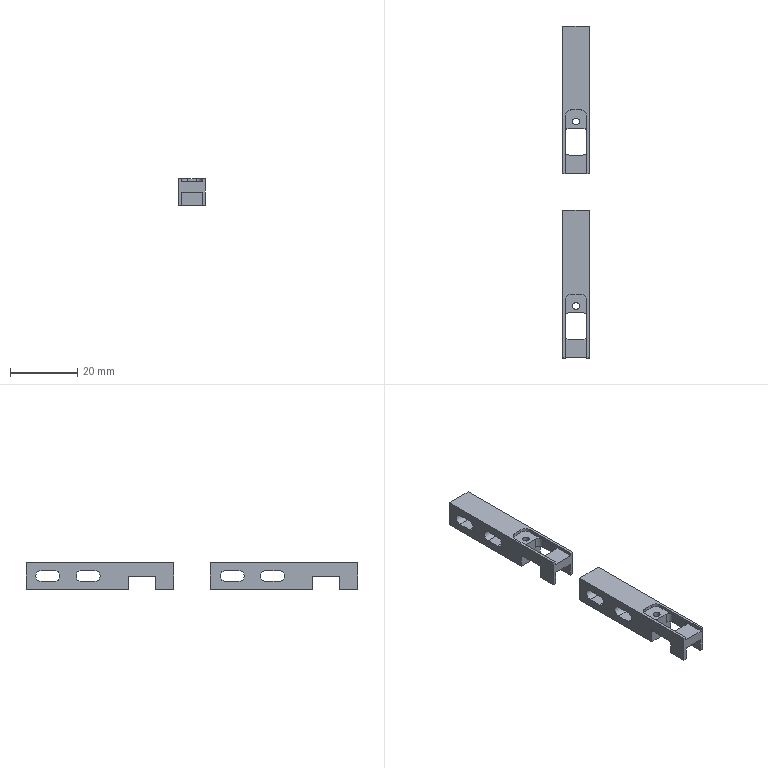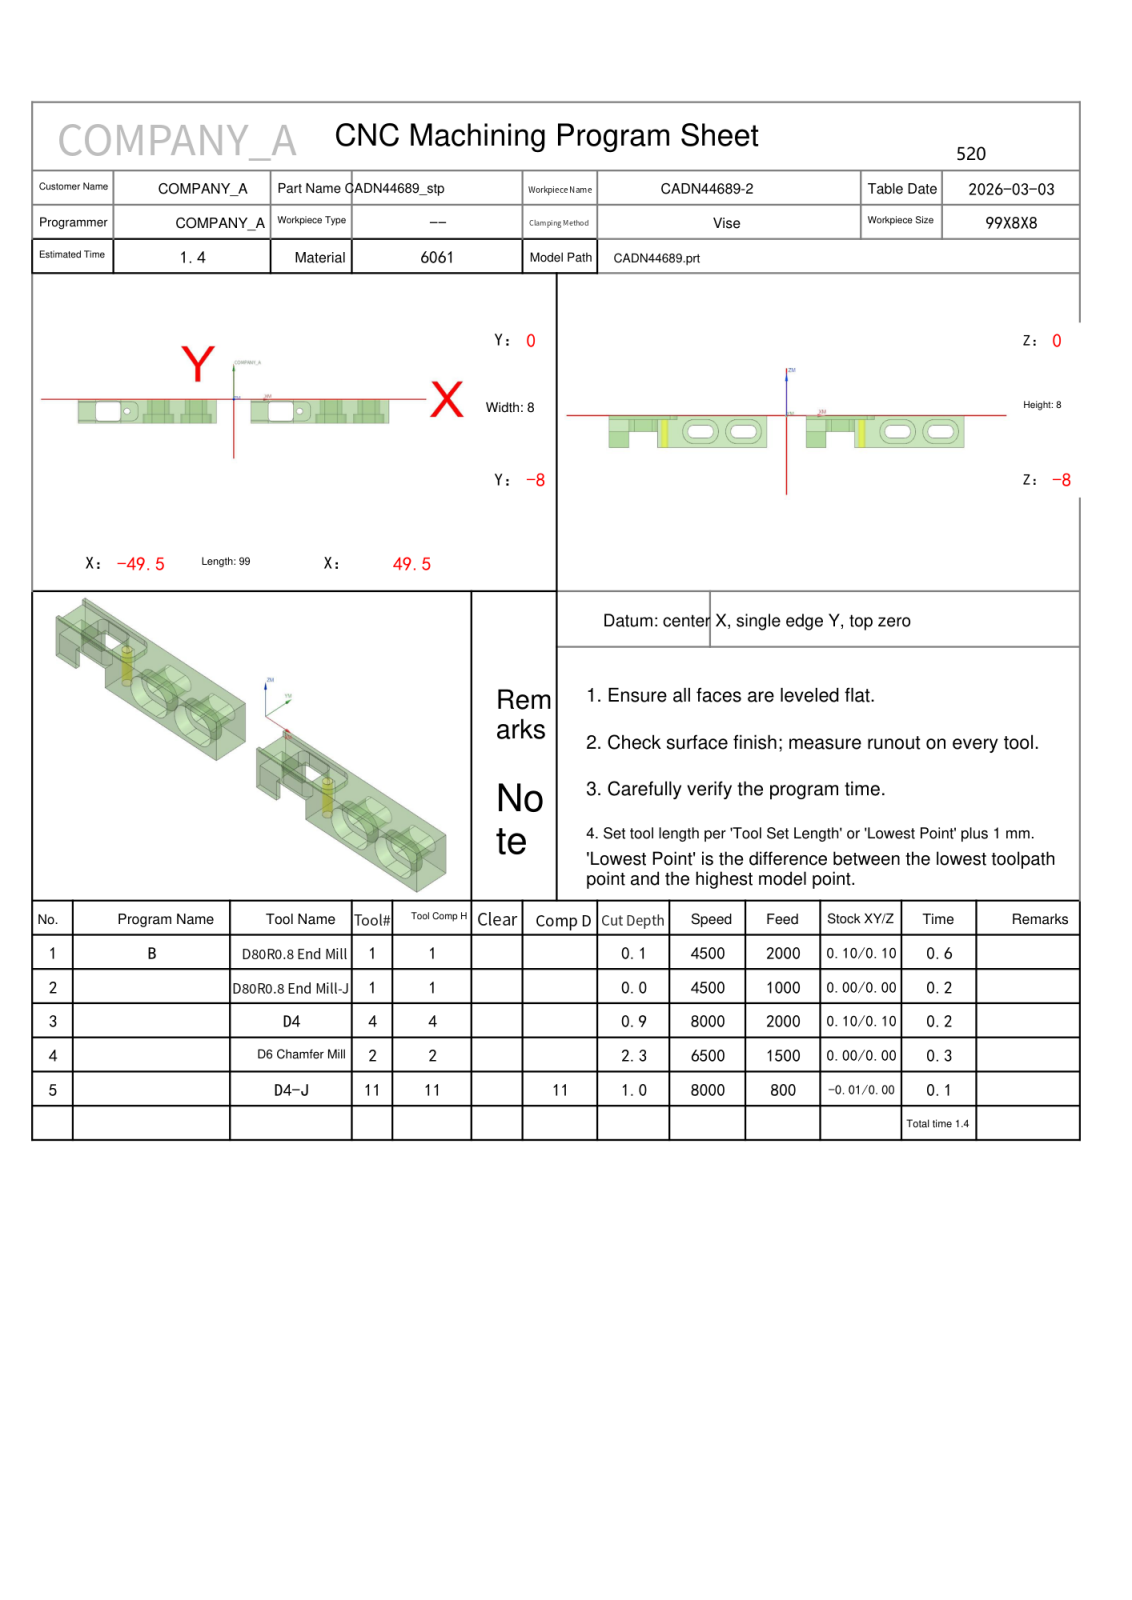NC program | NX | posted by the shop | part box 8 x 99 x 8 mm
Whole program:
%
O0001
(Machine time: 2.46 MIN)
(===Total Tool:4===)
(T1=D80R0.8 Indexable End Mill D=80.  R=0.8  D-  H01 Z=0.    )
(T4=D4      D=4.   R=0.   D-  H04 Z=-0.9  )
(T2=D6 Chamfer Mill   D=6.   R=0.   D-  H02 Z=-2.33 )
(T11=D4-J   D=4.   R=0.   D11 H11 Z=-1.   )
G80 G90 G17 G49 G40
G91 G28 Z0
M01
N1 T01 M06
(D80R0.8 Indexable End Mill  D=80. R=0.8 H=01 ce=0.10 di=0.10)
G00 G90 G54 X-101.597 Y-4. M03 S4500
G43 H01 Z50.
M08
Z5.62
G01 Z3.62 F2000.
X-89.597
X89.597
X101.597
Z5.62
G00 X-101.597
Z4.74
G01 Z2.74
X-89.597
X89.597
X101.597
Z4.74
G00 Z50.
X-101.597
Z3.86
G01 Z1.86
X-89.597
X89.597
X101.597
Z3.86
G00 Z50.
X-101.597
Z2.98
G01 Z.98
X-89.597
X89.597
X101.597
Z2.98
G00 Z50.
X-101.597
Z2.1
G01 Z.1
X-89.597
X89.597
X101.597
Z2.1
G00 Z50.
G91 G28 Z0.0
M05
M09
G91 G28 Z0.0
M01
N2 T01 M06
(D80R0.8 Indexable End Mill-J  D=80. R=0.8 H=01 ce=0.00 di=0.00)
G00 G90 G54 X-101.499 Y-4. M03 S4500
G43 H01 Z50.
M08
Z2.
G01 Z0.0 F1000.
X-89.499
X89.499
X101.499
Z2.
G00 Z50.
G91 G28 Z0.0
M05
M09
G91 G28 Z0.0
M01
N3 T04 M06
(D4  D=4. R=0. H=04 ce=0.10 di=0.10)
G00 G90 G54 X-54.6 Y-5.15 M03 S8000
G43 H04 Z11.8
M08
Z1.2
G01 Z-.3 F2000.
X-51.46
X-32.6
Y-2.85
X-51.46
X-54.6
Z1.2
G00 Y-5.15
Z.9
G01 Z-.6
X-51.46
X-32.6
Y-2.85
X-51.46
X-54.6
Z.9
G00 Y-5.15
Z.6
G01 Z-.9
X-51.46
X-32.6
Y-2.85
X-51.46
X-54.6
Z.6
G00 Z11.8
X.4 Y-5.15
Z1.2
G01 Z-.3
X3.54
X22.4
Y-2.85
X3.54
X.4
Z1.2
G00 Y-5.15
Z.9
G01 Z-.6
X3.54
X22.4
Y-2.85
X3.54
X.4
Z.9
G00 Y-5.15
Z.6
G01 Z-.9
X3.54
X22.4
Y-2.85
X3.54
X.4
Z.6
G00 Z11.8
G91 G28 Z0.0
M05
M09
G91 G28 Z0.0
M01
N4 T02 M06
(D6 Chamfer Mill  D=6. R=0. H=02 ce=0.00 di=0.10)
G00 G90 G54 X-34. Y-4. M03 S5000
G43 H02 Z50.
M08
G98 G81 X-34. Y-4. Z-2.325 R2. F150.
X21.
G80
G00 Z50.
G00 G90 X27.886 Y-8.827 M03 S6500
Z50.
Z.572
G01 Z-.8 F1500.
G03 X27.6 Y-8.627 I-1.286 J-1.532
G01 X27.554 Y-8.597
X27.5 Y-8.6
X5.5
G02 X4.9 Y-8. I0.0 J.6
G01 Y-7.25
G02 X5.5 Y-6.65 I.6 J0.0
G01 X22.5
G03 X23.9 Y-5.25 I0.0 J1.4
G01 Y-2.75
G03 X22.5 Y-1.35 I-1.4 J0.0
G01 X5.5
G02 X4.9 Y-.75 I0.0 J.6
G01 Y0.0
G02 X5.5 Y.6 I.6 J0.0
G01 X49.5
G02 X50.1 Y0.0 I0.0 J-.6
G01 Y-8.
G02 X49.5 Y-8.6 I-.6 J0.0
G01 X27.5
X27.446 Y-8.597
X27.4 Y-8.627
G03 X27.114 Y-8.827 I1. J-1.732
G01 Z.572
G00 Z10.
X-27.114
Z.572
G01 Z-.8
G03 X-27.4 Y-8.627 I-1.286 J-1.532
G01 X-27.446 Y-8.597
X-27.5 Y-8.6
X-49.5
G02 X-50.1 Y-8. I0.0 J.6
G01 Y-7.25
G02 X-49.5 Y-6.65 I.6 J0.0
G01 X-32.5
G03 X-31.1 Y-5.25 I0.0 J1.4
G01 Y-2.75
G03 X-32.5 Y-1.35 I-1.4 J0.0
G01 X-49.5
G02 X-50.1 Y-.75 I0.0 J.6
G01 Y0.0
G02 X-49.5 Y.6 I.6 J0.0
G01 X-5.5
G02 X-4.9 Y0.0 I0.0 J-.6
G01 Y-8.
G02 X-5.5 Y-8.6 I-.6 J0.0
G01 X-27.5
X-27.554 Y-8.597
X-27.6 Y-8.627
G03 X-27.886 Y-8.827 I1. J-1.732
G01 Z.572
G00 Z2.2
X-36.6 Y-5.469
G01 Z-1.8
Y-2.531
Z2.2
G00 Z10.
X-50.1 Y-5.574
Z2.2
G01 Z-1.8
Y-2.426
Z2.2
G00 X-43.4 Y-2.531
G01 Z-1.8
Y-5.469
Z2.2
G00 Z10.
X11.6 Y-2.531
Z2.2
G01 Z-1.8
Y-5.469
Z2.2
G00 X4.9 Y-5.574
G01 Z-1.8
Y-2.426
Z2.2
G00 Z10.
X18.4 Y-5.469
Z2.2
G01 Z-1.8
Y-2.531
Z2.2
G00 Z50.
G91 G28 Z0.0
M05
M09
G91 G28 Z0.0
M01
N5 T11 M06
(D4-J  D=4. R=0. H=11 ce=-0.01 di=0.00)
G00 G90 G54 X-52.322 Y-4.389 M03 S8000
G43 H11 Z11.8
M08
Z0.0
G01 Z-1. F800.
G41 D11
X-52.29 Y-4.586
G03 X-51.5 Y-5.26 I.79 J.126
G01 X-32.5
X-32.494 Y-5.261
X-32.489 Y-5.257
X-32.49 Y-5.25
Y-2.75
X-32.489 Y-2.744
X-32.494 Y-2.739
X-32.5 Y-2.74
X-51.5
G03 X-52.29 Y-3.414 I0.0 J-.8
G01 G40 X-52.322 Y-3.611
Z0.0
G00 Z3.
X2.678 Y-4.389
Z0.0
G01 Z-1.
G41 D11
X2.71 Y-4.586
G03 X3.5 Y-5.26 I.79 J.126
G01 X22.5
X22.507 Y-5.261
X22.511 Y-5.257
X22.51 Y-5.25
Y-2.75
X22.511 Y-2.744
X22.507 Y-2.739
X22.5 Y-2.74
X3.5
G03 X2.71 Y-3.414 I0.0 J-.8
G01 G40 X2.678 Y-3.611
Z0.0
G00 Z11.8
M05
M09
G91 G28 Z0.0
G91 G28 Y0.0
M30
%